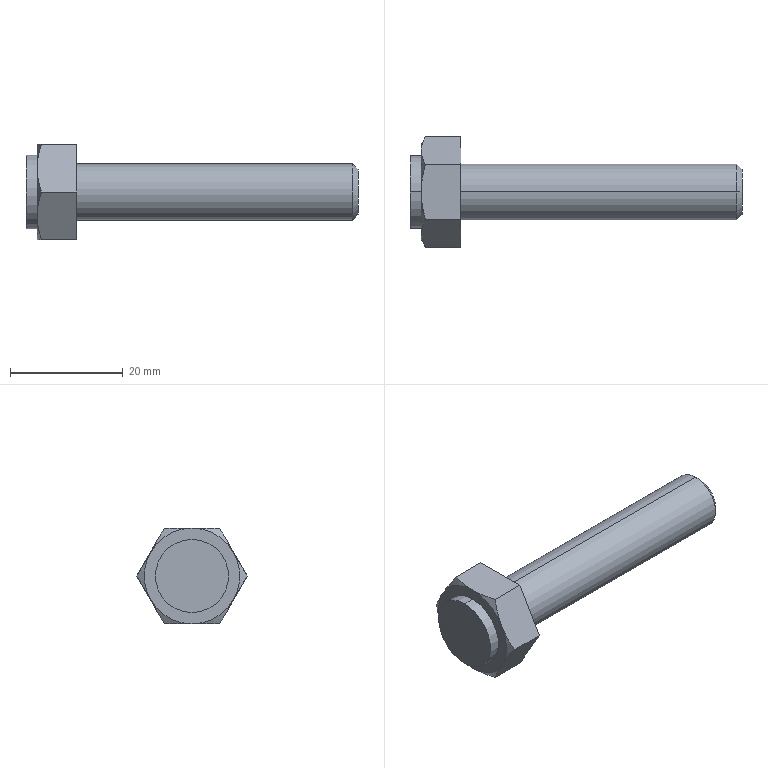Part | STEP file | 0244_Z_006_SUST10-50_1 | 1 solid | 22 faces | box 59 x 19.63 x 17 mm | volume 5927 mm3 | plane 10 | cone 8 | cylinder 4 | commonest cylinder face diameters 10 x2 13 x2